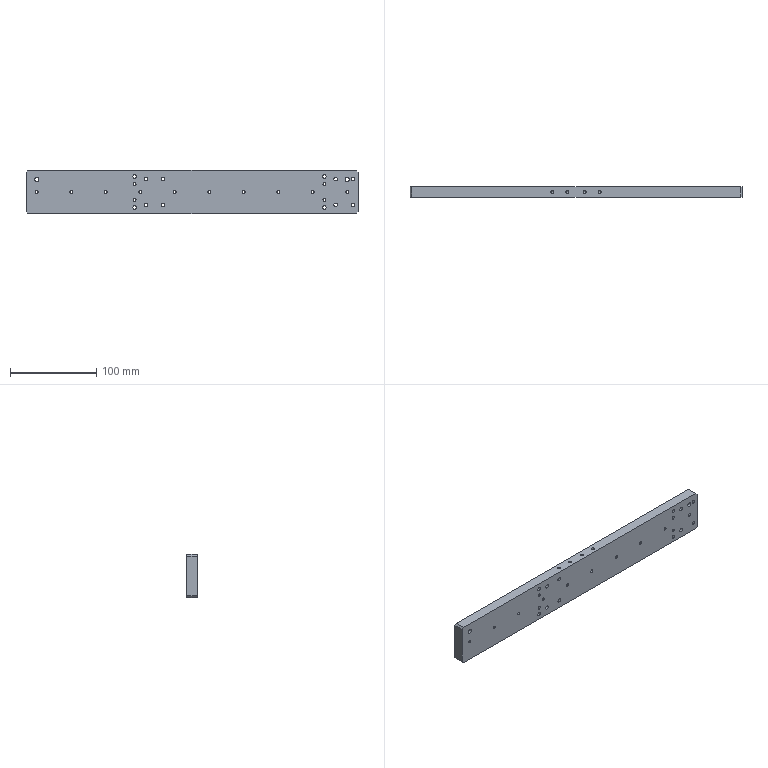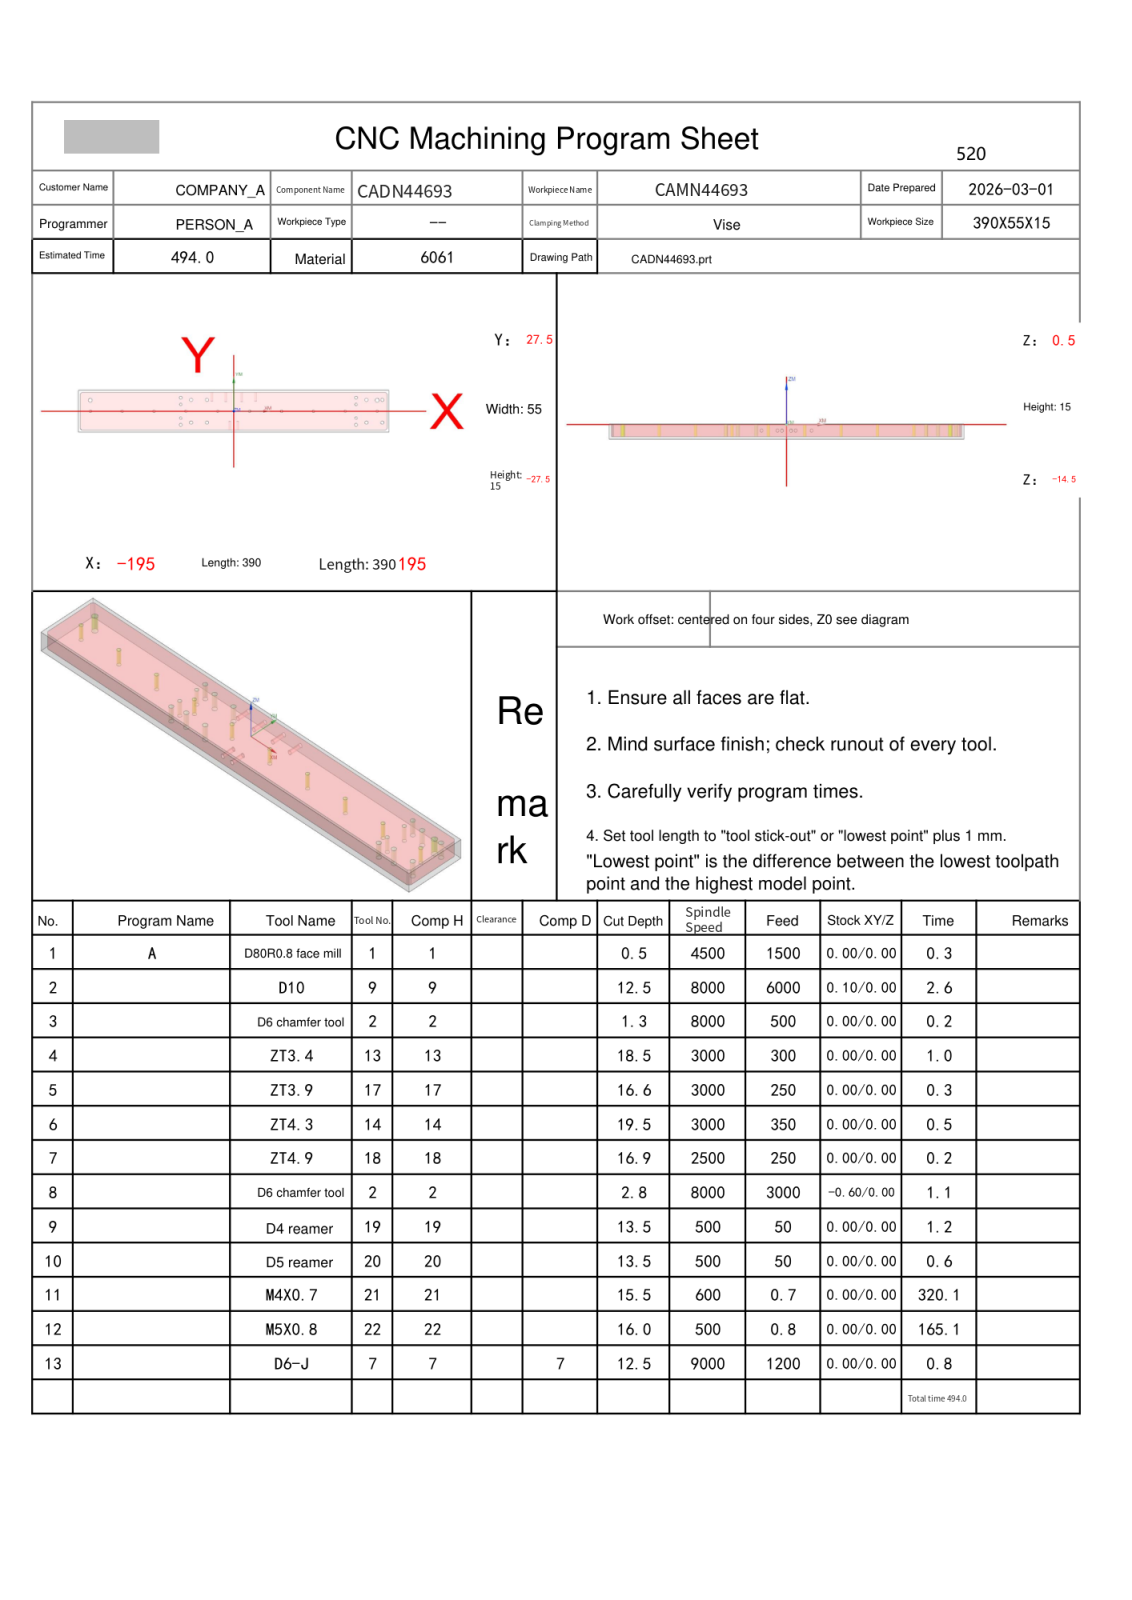NC program | NX | posted by the shop | part box 385 x 12 x 50 mm
Whole program:
%
O0001
(Machine time: 951.30 MIN)
(===Total Tool:12===)
(T1=D80R0.8 face mill D=80.  R=0.8  D-  H01 Z=0.    )
(T9=D10     D=10.  R=0.   D-  H09 Z=-12.  )
(T2=D6 chamfer tool   D=6.   R=0.   D-  H02 Z=-2.3  )
(T13=ZT3.4  D=3.4  DR_a=118 D-  H13 Z=-18.  )
(T17=ZT3.9  D=3.9  DR_a=120 D-  H17 Z=-16.13)
(T14=ZT4.3  D=4.3  DR_a=118 D-  H14 Z=-19.  )
(T18=ZT4.9  D=4.9  DR_a=120 D-  H18 Z=-16.41)
(T19=D4 reamer   D=4.   DR_a=180 D-  H19 Z=-13.  )
(T20=D5 reamer   D=5.   DR_a=180 D-  H20 Z=-13.  )
(T21=M4X0.7 D=3.3  DR_a=180 D-  H21 Z=-15.  )
(T22=M5X0.8 D=4.2  DR_a=180 D-  H22 Z=-15.5 )
(T7=D6-J    D=6.   R=0.   D7  H07 Z=-12.  )
G80 G90 G17 G49 G40
G91 G28 Z0
M01
N1 T01 M06
(D80R0.8 face mill  D=80. R=0.8 H=01 ce=0.00 di=0.00)
G00 G90 G54 X237.5 Y0.0 M03 S4500
G43 H01 Z50.
M08
Z2.
G01 Z0.0 F1500.
X232.5
X-232.5
X-237.5
Z2.
G00 Z50.
G91 G28 Z0.0
M05
M09
G91 G28 Z0.0
M01
N2 T09 M06
(D10  D=10. R=0. H=09 ce=0.10 di=0.00)
G00 G90 G54 X0.0 Y30.1 M03 S8000
G43 H09 Z50.
M08
Z.5
G01 X190.5 Z.334 F6000.
G02 X194.106 Y28.606 Z.331 I0.0 J-5.1
G01 X196.106 Y26.606 Z.328
G02 X197.6 Y23. Z.325 I-3.606 J-3.606
G01 Y-23. Z.285
G02 X196.106 Y-26.606 Z.281 I-5.1 J0.0
G01 X194.106 Y-28.606 Z.279
G02 X190.5 Y-30.1 Z.275 I-3.606 J3.606
G01 X-190.5 Z-.056
G02 X-194.106 Y-28.606 Z-.06 I0.0 J5.1
G01 X-196.106 Y-26.606 Z-.062
G02 X-197.6 Y-23. Z-.066 I3.606 J3.606
G01 Y23. Z-.106
G02 X-196.106 Y26.606 Z-.109 I5.1 J0.0
G01 X-194.106 Y28.606 Z-.112
G02 X-190.5 Y30.1 Z-.115 I3.606 J-3.606
G01 X190.5 Z-.447
G02 X194.106 Y28.606 Z-.451 I0.0 J-5.1
G01 X196.106 Y26.606 Z-.453
G02 X197.6 Y23. Z-.457 I-3.606 J-3.606
G01 Y-23. Z-.497
G02 X196.106 Y-26.606 Z-.5 I-5.1 J0.0
G01 X194.106 Y-28.606 Z-.503
G02 X190.5 Y-30.1 Z-.506 I-3.606 J3.606
G01 X-190.5 Z-.838
G02 X-194.106 Y-28.606 Z-.841 I0.0 J5.1
G01 X-196.106 Y-26.606 Z-.844
G02 X-197.6 Y-23. Z-.847 I3.606 J3.606
G01 Y23. Z-.887
G02 X-196.106 Y26.606 Z-.891 I5.1 J0.0
G01 X-194.106 Y28.606 Z-.893
G02 X-190.5 Y30.1 Z-.897 I3.606 J-3.606
G01 X190.5 Z-1.228
G02 X194.106 Y28.606 Z-1.232 I0.0 J-5.1
G01 X196.106 Y26.606 Z-1.234
G02 X197.6 Y23. Z-1.238 I-3.606 J-3.606
G01 Y-23. Z-1.278
G02 X196.106 Y-26.606 Z-1.281 I-5.1 J0.0
G01 X194.106 Y-28.606 Z-1.284
G02 X190.5 Y-30.1 Z-1.287 I-3.606 J3.606
G01 X-190.5 Z-1.619
G02 X-194.106 Y-28.606 Z-1.622 I0.0 J5.1
G01 X-196.106 Y-26.606 Z-1.625
G02 X-197.6 Y-23. Z-1.628 I3.606 J3.606
G01 Y23. Z-1.668
G02 X-196.106 Y26.606 Z-1.672 I5.1 J0.0
G01 X-194.106 Y28.606 Z-1.674
G02 X-190.5 Y30.1 Z-1.678 I3.606 J-3.606
G01 X190.5 Z-2.01
G02 X194.106 Y28.606 Z-2.013 I0.0 J-5.1
G01 X196.106 Y26.606 Z-2.016
G02 X197.6 Y23. Z-2.019 I-3.606 J-3.606
G01 Y-23. Z-2.059
G02 X196.106 Y-26.606 Z-2.063 I-5.1 J0.0
G01 X194.106 Y-28.606 Z-2.065
G02 X190.5 Y-30.1 Z-2.069 I-3.606 J3.606
G01 X-190.5 Z-2.4
G02 X-194.106 Y-28.606 Z-2.404 I0.0 J5.1
G01 X-196.106 Y-26.606 Z-2.406
G02 X-197.6 Y-23. Z-2.41 I3.606 J3.606
G01 Y23. Z-2.45
G02 X-196.106 Y26.606 Z-2.453 I5.1 J0.0
G01 X-194.106 Y28.606 Z-2.456
G02 X-190.5 Y30.1 Z-2.459 I3.606 J-3.606
G01 X190.5 Z-2.791
G02 X194.106 Y28.606 Z-2.794 I0.0 J-5.1
G01 X196.106 Y26.606 Z-2.797
G02 X197.6 Y23. Z-2.8 I-3.606 J-3.606
G01 Y-23. Z-2.84
G02 X196.106 Y-26.606 Z-2.844 I-5.1 J0.0
G01 X194.106 Y-28.606 Z-2.846
G02 X190.5 Y-30.1 Z-2.85 I-3.606 J3.606
G01 X-190.5 Z-3.181
G02 X-194.106 Y-28.606 Z-3.185 I0.0 J5.1
G01 X-196.106 Y-26.606 Z-3.187
G02 X-197.6 Y-23. Z-3.191 I3.606 J3.606
G01 Y23. Z-3.231
G02 X-196.106 Y26.606 Z-3.234 I5.1 J0.0
G01 X-194.106 Y28.606 Z-3.237
G02 X-190.5 Y30.1 Z-3.24 I3.606 J-3.606
G01 X190.5 Z-3.572
G02 X194.106 Y28.606 Z-3.576 I0.0 J-5.1
G01 X196.106 Y26.606 Z-3.578
G02 X197.6 Y23. Z-3.582 I-3.606 J-3.606
G01 Y-23. Z-3.622
G02 X196.106 Y-26.606 Z-3.625 I-5.1 J0.0
G01 X194.106 Y-28.606 Z-3.628
G02 X190.5 Y-30.1 Z-3.631 I-3.606 J3.606
G01 X-190.5 Z-3.963
G02 X-194.106 Y-28.606 Z-3.966 I0.0 J5.1
G01 X-196.106 Y-26.606 Z-3.969
G02 X-197.6 Y-23. Z-3.972 I3.606 J3.606
G01 Y23. Z-4.012
G02 X-196.106 Y26.606 Z-4.016 I5.1 J0.0
G01 X-194.106 Y28.606 Z-4.018
G02 X-190.5 Y30.1 Z-4.022 I3.606 J-3.606
G01 X190.5 Z-4.353
G02 X194.106 Y28.606 Z-4.357 I0.0 J-5.1
G01 X196.106 Y26.606 Z-4.359
G02 X197.6 Y23. Z-4.363 I-3.606 J-3.606
G01 Y-23. Z-4.403
G02 X196.106 Y-26.606 Z-4.406 I-5.1 J0.0
G01 X194.106 Y-28.606 Z-4.409
G02 X190.5 Y-30.1 Z-4.412 I-3.606 J3.606
G01 X-190.5 Z-4.744
G02 X-194.106 Y-28.606 Z-4.747 I0.0 J5.1
G01 X-196.106 Y-26.606 Z-4.75
G02 X-197.6 Y-23. Z-4.753 I3.606 J3.606
G01 Y23. Z-4.793
G02 X-196.106 Y26.606 Z-4.797 I5.1 J0.0
G01 X-194.106 Y28.606 Z-4.799
G02 X-190.5 Y30.1 Z-4.803 I3.606 J-3.606
G01 X190.5 Z-5.135
G02 X194.106 Y28.606 Z-5.138 I0.0 J-5.1
G01 X196.106 Y26.606 Z-5.141
G02 X197.6 Y23. Z-5.144 I-3.606 J-3.606
G01 Y-23. Z-5.184
G02 X196.106 Y-26.606 Z-5.188 I-5.1 J0.0
G01 X194.106 Y-28.606 Z-5.19
G02 X190.5 Y-30.1 Z-5.194 I-3.606 J3.606
G01 X-190.5 Z-5.525
G02 X-194.106 Y-28.606 Z-5.529 I0.0 J5.1
G01 X-196.106 Y-26.606 Z-5.531
G02 X-197.6 Y-23. Z-5.535 I3.606 J3.606
G01 Y23. Z-5.575
G02 X-196.106 Y26.606 Z-5.578 I5.1 J0.0
G01 X-194.106 Y28.606 Z-5.581
G02 X-190.5 Y30.1 Z-5.584 I3.606 J-3.606
G01 X190.5 Z-5.916
G02 X194.106 Y28.606 Z-5.919 I0.0 J-5.1
G01 X196.106 Y26.606 Z-5.922
G02 X197.6 Y23. Z-5.925 I-3.606 J-3.606
G01 Y-23. Z-5.965
G02 X196.106 Y-26.606 Z-5.969 I-5.1 J0.0
G01 X194.106 Y-28.606 Z-5.971
G02 X190.5 Y-30.1 Z-5.975 I-3.606 J3.606
G01 X-190.5 Z-6.306
G02 X-194.106 Y-28.606 Z-6.31 I0.0 J5.1
G01 X-196.106 Y-26.606 Z-6.312
G02 X-197.6 Y-23. Z-6.316 I3.606 J3.606
G01 Y23. Z-6.356
G02 X-196.106 Y26.606 Z-6.359 I5.1 J0.0
G01 X-194.106 Y28.606 Z-6.362
G02 X-190.5 Y30.1 Z-6.365 I3.606 J-3.606
G01 X190.5 Z-6.697
G02 X194.106 Y28.606 Z-6.701 I0.0 J-5.1
G01 X196.106 Y26.606 Z-6.703
G02 X197.6 Y23. Z-6.707 I-3.606 J-3.606
G01 Y-23. Z-6.747
G02 X196.106 Y-26.606 Z-6.75 I-5.1 J0.0
G01 X194.106 Y-28.606 Z-6.753
G02 X190.5 Y-30.1 Z-6.756 I-3.606 J3.606
G01 X-190.5 Z-7.088
G02 X-194.106 Y-28.606 Z-7.091 I0.0 J5.1
G01 X-196.106 Y-26.606 Z-7.094
G02 X-197.6 Y-23. Z-7.097 I3.606 J3.606
G01 Y23. Z-7.137
G02 X-196.106 Y26.606 Z-7.141 I5.1 J0.0
G01 X-194.106 Y28.606 Z-7.143
G02 X-190.5 Y30.1 Z-7.147 I3.606 J-3.606
G01 X190.5 Z-7.478
G02 X194.106 Y28.606 Z-7.482 I0.0 J-5.1
G01 X196.106 Y26.606 Z-7.484
G02 X197.6 Y23. Z-7.488 I-3.606 J-3.606
G01 Y-23. Z-7.528
G02 X196.106 Y-26.606 Z-7.531 I-5.1 J0.0
G01 X194.106 Y-28.606 Z-7.534
G02 X190.5 Y-30.1 Z-7.537 I-3.606 J3.606
G01 X-190.5 Z-7.869
G02 X-194.106 Y-28.606 Z-7.872 I0.0 J5.1
G01 X-196.106 Y-26.606 Z-7.875
G02 X-197.6 Y-23. Z-7.878 I3.606 J3.606
G01 Y23. Z-7.918
G02 X-196.106 Y26.606 Z-7.922 I5.1 J0.0
G01 X-194.106 Y28.606 Z-7.924
G02 X-190.5 Y30.1 Z-7.928 I3.606 J-3.606
G01 X190.5 Z-8.26
G02 X194.106 Y28.606 Z-8.263 I0.0 J-5.1
G01 X196.106 Y26.606 Z-8.266
G02 X197.6 Y23. Z-8.269 I-3.606 J-3.606
G01 Y-23. Z-8.309
G02 X196.106 Y-26.606 Z-8.313 I-5.1 J0.0
G01 X194.106 Y-28.606 Z-8.315
G02 X190.5 Y-30.1 Z-8.319 I-3.606 J3.606
G01 X-190.5 Z-8.65
G02 X-194.106 Y-28.606 Z-8.654 I0.0 J5.1
G01 X-196.106 Y-26.606 Z-8.656
G02 X-197.6 Y-23. Z-8.66 I3.606 J3.606
G01 Y23. Z-8.7
G02 X-196.106 Y26.606 Z-8.703 I5.1 J0.0
G01 X-194.106 Y28.606 Z-8.706
G02 X-190.5 Y30.1 Z-8.709 I3.606 J-3.606
G01 X190.5 Z-9.041
G02 X194.106 Y28.606 Z-9.044 I0.0 J-5.1
G01 X196.106 Y26.606 Z-9.047
G02 X197.6 Y23. Z-9.05 I-3.606 J-3.606
G01 Y-23. Z-9.09
G02 X196.106 Y-26.606 Z-9.094 I-5.1 J0.0
G01 X194.106 Y-28.606 Z-9.096
G02 X190.5 Y-30.1 Z-9.1 I-3.606 J3.606
G01 X-190.5 Z-9.431
G02 X-194.106 Y-28.606 Z-9.435 I0.0 J5.1
G01 X-196.106 Y-26.606 Z-9.437
G02 X-197.6 Y-23. Z-9.441 I3.606 J3.606
G01 Y23. Z-9.481
G02 X-196.106 Y26.606 Z-9.484 I5.1 J0.0
G01 X-194.106 Y28.606 Z-9.487
G02 X-190.5 Y30.1 Z-9.49 I3.606 J-3.606
G01 X190.5 Z-9.822
G02 X194.106 Y28.606 Z-9.826 I0.0 J-5.1
G01 X196.106 Y26.606 Z-9.828
G02 X197.6 Y23. Z-9.832 I-3.606 J-3.606
G01 Y-23. Z-9.872
G02 X196.106 Y-26.606 Z-9.875 I-5.1 J0.0
G01 X194.106 Y-28.606 Z-9.878
G02 X190.5 Y-30.1 Z-9.881 I-3.606 J3.606
G01 X-190.5 Z-10.213
G02 X-194.106 Y-28.606 Z-10.216 I0.0 J5.1
G01 X-196.106 Y-26.606 Z-10.219
G02 X-197.6 Y-23. Z-10.222 I3.606 J3.606
G01 Y23. Z-10.262
G02 X-196.106 Y26.606 Z-10.266 I5.1 J0.0
G01 X-194.106 Y28.606 Z-10.268
G02 X-190.5 Y30.1 Z-10.272 I3.606 J-3.606
G01 X190.5 Z-10.603
G02 X194.106 Y28.606 Z-10.607 I0.0 J-5.1
G01 X196.106 Y26.606 Z-10.609
G02 X197.6 Y23. Z-10.613 I-3.606 J-3.606
G01 Y-23. Z-10.653
G02 X196.106 Y-26.606 Z-10.656 I-5.1 J0.0
G01 X194.106 Y-28.606 Z-10.659
G02 X190.5 Y-30.1 Z-10.662 I-3.606 J3.606
G01 X-190.5 Z-10.994
G02 X-194.106 Y-28.606 Z-10.997 I0.0 J5.1
G01 X-196.106 Y-26.606 Z-11.
G02 X-197.6 Y-23. Z-11.003 I3.606 J3.606
G01 Y23. Z-11.043
G02 X-196.106 Y26.606 Z-11.047 I5.1 J0.0
G01 X-194.106 Y28.606 Z-11.049
G02 X-190.5 Y30.1 Z-11.053 I3.606 J-3.606
G01 X190.5 Z-11.385
G02 X194.106 Y28.606 Z-11.388 I0.0 J-5.1
G01 X196.106 Y26.606 Z-11.391
G02 X197.6 Y23. Z-11.394 I-3.606 J-3.606
G01 Y-23. Z-11.434
G02 X196.106 Y-26.606 Z-11.438 I-5.1 J0.0
G01 X194.106 Y-28.606 Z-11.44
G02 X190.5 Y-30.1 Z-11.444 I-3.606 J3.606
G01 X-190.5 Z-11.775
G02 X-194.106 Y-28.606 Z-11.779 I0.0 J5.1
G01 X-196.106 Y-26.606 Z-11.781
G02 X-197.6 Y-23. Z-11.785 I3.606 J3.606
G01 Y23. Z-11.825
G02 X-196.106 Y26.606 Z-11.828 I5.1 J0.0
G01 X-194.106 Y28.606 Z-11.831
G02 X-190.5 Y30.1 Z-11.834 I3.606 J-3.606
G01 X0.0 Z-12.
X190.5
G02 X194.106 Y28.606 I0.0 J-5.1
G01 X196.106 Y26.606
G02 X197.6 Y23. I-3.606 J-3.606
G01 Y-23.
G02 X196.106 Y-26.606 I-5.1 J0.0
G01 X194.106 Y-28.606
G02 X190.5 Y-30.1 I-3.606 J3.606
G01 X-190.5
G02 X-194.106 Y-28.606 I0.0 J5.1
G01 X-196.106 Y-26.606
G02 X-197.6 Y-23. I3.606 J3.606
G01 Y23.
G02 X-196.106 Y26.606 I5.1 J0.0
G01 X-194.106 Y28.606
G02 X-190.5 Y30.1 I3.606 J-3.606
G01 X0.0
X.5
Z-11.
G00 Z50.
G91 G28 Z0.0
M05
M09
G91 G28 Z0.0
M01
N3 T02 M06
(D6 chamfer tool  D=6. R=0. H=02 ce=0.00 di=0.00)
G00 G90 G54 X-180. Y14.5 M03 S8000
G43 H02 Z50.
M08
G98 G81 X-180. Y14.5 Z-.8 R1. F500.
Y0.0
X-140.
X-100.
X-66.5 Y-9.
Y-18.
X-53.5 Y-15.
X-60. Y0.0
X-66.5 Y9.
Y18.
X-53.5 Y15.
X-33.5
Y-15.
X-20. Y0.0
X20.
X60.
X100.
X140.
X153.5 Y9.
Y18.
X166.5 Y15.
X180. Y14.5
X186.5 Y15.
X180. Y0.0
X186.5 Y-15.
X166.5
X153.5 Y-18.
Y-9.
G80
G00 Z50.
G91 G28 Z0.0
M05
M09
G91 G28 Z0.0
M01
N4 T13 M06
(ZT3.4 D=3.4 DR_a=118 H=13)
G00 G90 G54 X180. Y0.0 M03 S3000
G43 H13 Z50.
M08
G98 G83 X180. Y0.0 Z-18. R1. F300. Q2.
X153.5 Y9.
Y-9.
X140. Y0.0
X100.
X60.
X20.
X-20.
X-60.
X-66.5 Y-9.
Y9.
X-100. Y0.0
X-140.
X-180.
G80
G00 Z50.
G91 G28 Z0.0
M05
M09
G91 G28 Z0.0
M01
N5 T17 M06
(ZT3.9 D=3.9 DR_a=120 H=17)
G00 G90 G54 X153.5 Y-18. M03 S3000
G43 H17 Z50.
M08
G98 G83 X153.5 Y-18. Z-16.126 R1. F250. Q2.
Y18.
X-66.5
Y-18.
G80
G00 Z50.
G91 G28 Z0.0
M05
M09
G91 G28 Z0.0
M01
N6 T14 M06
(ZT4.3 D=4.3 DR_a=118 H=14)
G00 G90 G54 X166.5 Y15. M03 S3000
G43 H14 Z50.
M08
G98 G83 X166.5 Y15. Z-19. R1. F350. Q3.
X186.5
Y-15.
X166.5
X-33.5
X-53.5
Y15.
X-33.5
G80
G00 Z50.
G91 G28 Z0.0
M05
M09
G91 G28 Z0.0
M01
N7 T18 M06
(ZT4.9 D=4.9 DR_a=120 H=18)
G00 G90 G54 X-180. Y14.5 M03 S2500
G43 H18 Z50.
M08
G98 G83 X-180. Y14.5 Z-16.415 R1. F250. Q2.
X180.
G80
G00 Z50.
G91 G28 Z0.0
M05
M09
G91 G28 Z0.0
M01
N8 T02 M06
(D6 chamfer tool  D=6. R=0. H=02 ce=0.00 di=0.00)
G00 G90 G54 X.25 Y-27.128 M03 S8000
G43 H02 Z50.
M08
Z2.099
G01 Z-1.5 F3000.
G03 X.33 Y-26.828 I-.52 J.3
X.03 Y-26.308 I-.6 J0.0
G01 X0.0 Y-26.3
X-190.5
X-190.754 Y-26.275
X-190.997 Y-26.201
X-191.222 Y-26.081
X-191.419 Y-25.919
X-193.419 Y-23.919
X-193.581 Y-23.722
X-193.701 Y-23.497
X-193.775 Y-23.254
X-193.8 Y-23.
Y23.
X-193.775 Y23.254
X-193.701 Y23.497
X-193.581 Y23.722
X-193.419 Y23.919
X-191.419 Y25.919
X-191.222 Y26.081
X-190.997 Y26.201
X-190.754 Y26.275
X-190.5 Y26.3
X190.5
X190.754 Y26.275
X190.997 Y26.201
X191.222 Y26.081
X191.419 Y25.919
X193.419 Y23.919
X193.581 Y23.722
X193.701 Y23.497
X193.775 Y23.254
X193.8 Y23.
Y-23.
X193.775 Y-23.254
X193.701 Y-23.497
X193.581 Y-23.722
X193.419 Y-23.919
X191.419 Y-25.919
X191.222 Y-26.081
X190.997 Y-26.201
X190.754 Y-26.275
X190.5 Y-26.3
X0.0
X-.03 Y-26.308
G03 X-.33 Y-26.828 I.3 J-.52
X-.25 Y-27.128 I.6 J0.0
G01 Z2.099
G00 Z50.
G00 G90 X180. Y0.0 M03 S8000
Z50.
G98 G81 X180. Y0.0 Z-2.2 R3. F500.
X153.5 Y9.
Y-9.
X140. Y0.0
X100.
X60.
X20.
X-20.
X-60.
X-66.5 Y-9.
Y9.
X-100. Y0.0
X-140.
X-180.
G80
G00 Z50.
G00 G90 X153.5 Y-18. M03 S8000
Z50.
G98 G81 X153.5 Y-18. Z-2.3 R3. F500.
Y18.
X-66.5
Y-18.
G80
G00 Z50.
G00 G90 X165.806 Y14.907 M03 S8000
Z50.
Z-.5
G01 Z-1. F500.
X165. Y14.8
G03 X166.5 Y13.3 I1.5 J0.0
X168.2 Y15. I0.0 J1.7
X166.5 Y16.7 I-1.7 J0.0
X164.8 Y15. I0.0 J-1.7
X166.5 Y13.3 I1.7 J0.0
X168. Y14.8 I0.0 J1.5
G01 X167.194 Y14.907
Z-.5
G00 Z50.
X185.806
Z-.5
G01 Z-1.
X185. Y14.8
G03 X186.5 Y13.3 I1.5 J0.0
X188.2 Y15. I0.0 J1.7
X186.5 Y16.7 I-1.7 J0.0
X184.8 Y15. I0.0 J-1.7
X186.5 Y13.3 I1.7 J0.0
X188. Y14.8 I0.0 J1.5
G01 X187.194 Y14.907
Z-.5
G00 Z50.
X185.806 Y-15.093
Z-.5
G01 Z-1.
X185. Y-15.2
G03 X186.5 Y-16.7 I1.5 J0.0
X188.2 Y-15. I0.0 J1.7
X186.5 Y-13.3 I-1.7 J0.0
X184.8 Y-15. I0.0 J-1.7
X186.5 Y-16.7 I1.7 J0.0
X188. Y-15.2 I0.0 J1.5
G01 X187.194 Y-15.093
Z-.5
G00 Z50.
X165.806
Z-.5
G01 Z-1.
X165. Y-15.2
G03 X166.5 Y-16.7 I1.5 J0.0
X168.2 Y-15. I0.0 J1.7
X166.5 Y-13.3 I-1.7 J0.0
X164.8 Y-15. I0.0 J-1.7
X166.5 Y-16.7 I1.7 J0.0
X168. Y-15.2 I0.0 J1.5
G01 X167.194 Y-15.093
Z-.5
G00 Z50.
X-34.194
Z-.5
G01 Z-1.
X-35. Y-15.2
G03 X-33.5 Y-16.7 I1.5 J0.0
X-31.8 Y-15. I0.0 J1.7
X-33.5 Y-13.3 I-1.7 J0.0
X-35.2 Y-15. I0.0 J-1.7
X-33.5 Y-16.7 I1.7 J0.0
X-32. Y-15.2 I0.0 J1.5
G01 X-32.806 Y-15.093
Z-.5
G00 Z50.
X-54.194
Z-.5
G01 Z-1.
X-55. Y-15.2
G03 X-53.5 Y-16.7 I1.5 J0.0
X-51.8 Y-15. I0.0 J1.7
X-53.5 Y-13.3 I-1.7 J0.0
X-55.2 Y-15. I0.0 J-1.7
X-53.5 Y-16.7 I1.7 J0.0
X-52. Y-15.2 I0.0 J1.5
G01 X-52.806 Y-15.093
Z-.5
G00 Z50.
X-54.194 Y14.907
Z-.5
G01 Z-1.
X-55. Y14.8
G03 X-53.5 Y13.3 I1.5 J0.0
X-51.8 Y15. I0.0 J1.7
X-53.5 Y16.7 I-1.7 J0.0
X-55.2 Y15. I0.0 J-1.7
X-53.5 Y13.3 I1.7 J0.0
X-52. Y14.8 I0.0 J1.5
G01 X-52.806 Y14.907
Z-.5
G00 Z50.
X-34.194
Z-.5
G01 Z-1.
X-35. Y14.8
G03 X-33.5 Y13.3 I1.5 J0.0
X-31.8 Y15. I0.0 J1.7
X-33.5 Y16.7 I-1.7 J0.0
X-35.2 Y15. I0.0 J-1.7
X-33.5 Y13.3 I1.7 J0.0
X-32. Y14.8 I0.0 J1.5
G01 X-32.806 Y14.907
Z-.5
G00 Z50.
G00 G90 X-179.216 Y14.657 M03 S8000
Z50.
Z-.5
G01 Z-1. F500.
X-178.5 Y14.8
G03 X-180. Y16.3 I-1.5 J0.0
X-181.8 Y14.5 I0.0 J-1.8
X-180. Y12.7 I1.8 J0.0
X-178.2 Y14.5 I0.0 J1.8
X-180. Y16.3 I-1.8 J0.0
X-181.5 Y14.8 I0.0 J-1.5
G01 X-180.784 Y14.657
Z-.5
G00 Z50.
X180.784
Z-.5
G01 Z-1.
X181.5 Y14.8
G03 X180. Y16.3 I-1.5 J0.0
X178.2 Y14.5 I0.0 J-1.8
X180. Y12.7 I1.8 J0.0
X181.8 Y14.5 I0.0 J1.8
X180. Y16.3 I-1.8 J0.0
X178.5 Y14.8 I0.0 J-1.5
G01 X179.216 Y14.657
Z-.5
G00 Z50.
G91 G28 Z0.0
M05
M09
G91 G28 Z0.0
M01
N9 T19 M06
(D4 reamer D=4. DR_a=180 H=19)
G00 G90 G54 X153.5 Y-18. M03 S500
G43 H19 Z50.
M08
G98 G81 X153.5 Y-18. Z-13. R1. F50.
Y18.
X-66.5
Y-18.
G80
G00 Z50.
G91 G28 Z0.0
M05
M09
G91 G28 Z0.0
M01
N10 T20 M06
(D5 reamer D=5. DR_a=180 H=20)
G00 G90 G54 X-180. Y14.5 M03 S500
G43 H20 Z50.
M08
G98 G81 X-180. Y14.5 Z-13. R1. F50.
X180.
G80
G00 Z50.
G91 G28 Z0.0
M05
M09
G91 G28 Z0.0
M01
N11 T21 M06
(M4X0.7 D=3.3 DR_a=180 H=21)
G00 G90 G54 X180. Y0.0 M03 S600
G43 H21 Z50.
M08
G95
G98 G84 X180. Y0.0 Z-15. R1. F.7 Q4.
X153.5 Y9.
Y-9.
X140. Y0.0
X100.
X60.
X20.
X-20.
X-60.
X-66.5 Y-9.
Y9.
X-100. Y0.0
X-140.
X-180.
G80
G94
G00 Z50.
G91 G28 Z0.0
M05
M09
G91 G28 Z0.0
M01
N12 T22 M06
(M5X0.8 D=4.2 DR_a=180 H=22)
G00 G90 G54 X166.5 Y15. M03 S500
G43 H22 Z50.
M08
G95
G98 G84 X166.5 Y15. Z-15.5 R1. F.8 Q3.
X186.5
Y-15.
X166.5
X-33.5
X-53.5
Y15.
X-33.5
G80
G94
G00 Z50.
G91 G28 Z0.0
M05
M09
G91 G28 Z0.0
M01
N13 T07 M06
(D6-J  D=6. R=0. H=07 ce=0.00 di=0.00)
G00 G90 G54 X191.517 Y-29.073 M03 S9000
G43 H07 Z50.
M08
Z-11.5
G01 Z-12. F1200.
G41 D07
X191.492 Y-28.875
G03 X190.5 Y-28. I-.992 J-.125
G01 X-190.5
G02 X-192.621 Y-27.121 I0.0 J3.
G01 X-194.621 Y-25.121
G02 X-195.5 Y-23. I2.121 J2.121
G01 Y23.
G02 X-194.621 Y25.121 I3. J0.0
G01 X-192.621 Y27.121
G02 X-190.5 Y28. I2.121 J-2.121
G01 X190.5
G02 X192.621 Y27.121 I0.0 J-3.
G01 X194.621 Y25.121
G02 X195.5 Y23. I-2.121 J-2.121
G01 Y-23.
G02 X194.621 Y-25.121 I-3. J0.0
G01 X192.621 Y-27.121
G02 X190.5 Y-28. I-2.121 J2.121
G01 X190.
G03 X189. Y-29. I0.0 J-1.
G01 G40 Y-29.2
Z-11.5
G00 Z50.
M05
M09
G91 G28 Z0.0
G91 G28 Y0.0
M30
%